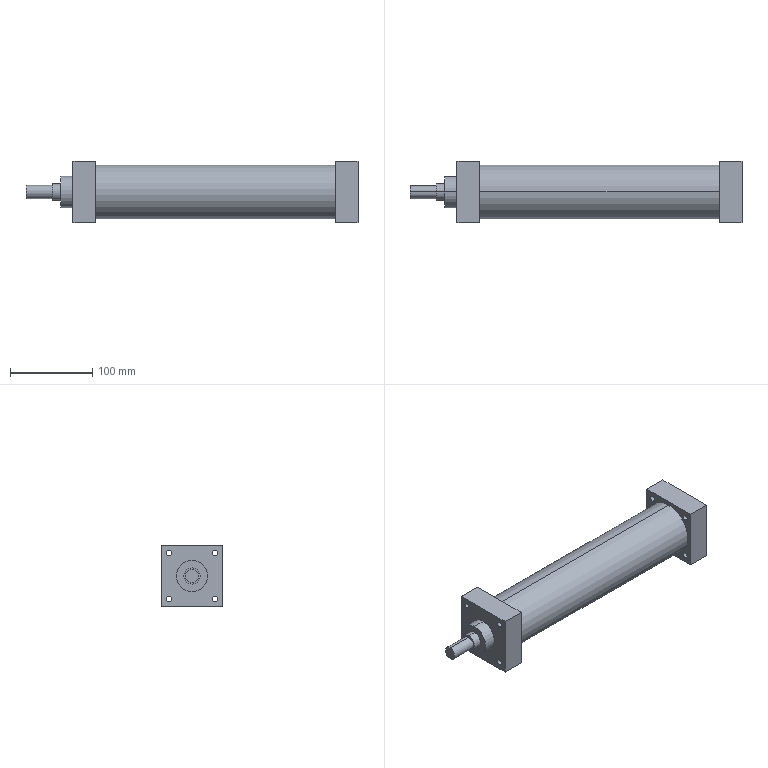Part | STEP file | PN_0029 (SC63X250) | 1 solid | 39 faces | box 403 x 75 x 75 mm | volume 1293600 mm3 | cylinder 24 | plane 15 | commonest cylinder face diameters 6.8 x16 16 x2 20 x2 38 x2 65 x2